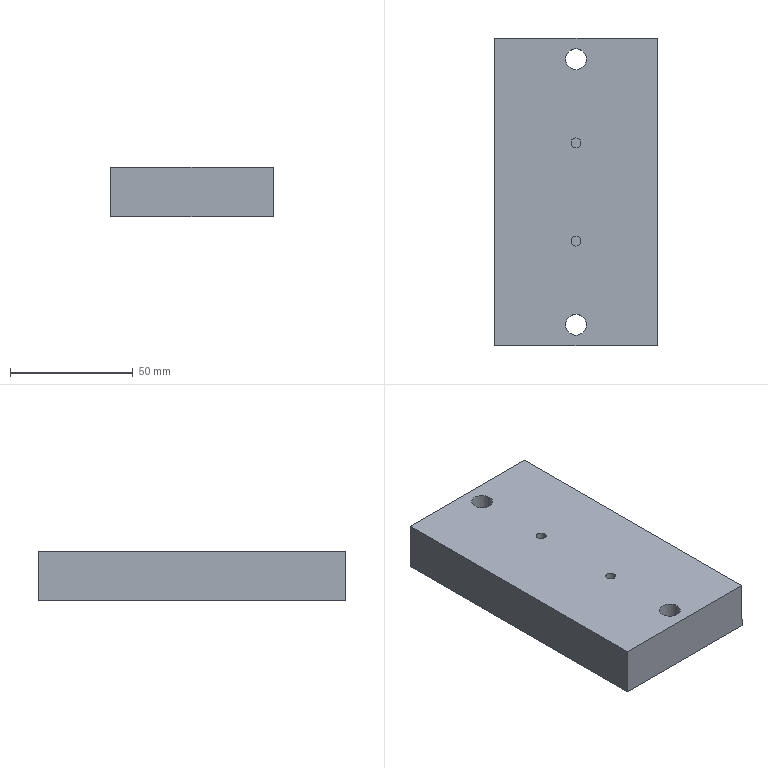NC program | NX | posted with a generic post | part box 65.936 x 125 x 20 mm
Lines 6200 to 6994 of 29196:
(PLANAR_MILL_2_COPY_COPY , TOOL : D10R0)
N12194 T10 M6
N12196 G54
N12198 G17 G0 G90 X-53.462 Y34.647 S4000 M3
N12200 G43 Z30. H10
N12202 G94 G1 Z-13.425 F5000.
N12204 G41 X-51. Y34.213 F1000. D10
N12206 X-45.
N12208 X45.
N12210 X51.
N12212 G40
N12214 X53.462 Y34.647
N12216 G0 Z5.
N12218 X-53.462
N12220 G1 Z-13.425 F5000.
N12222 G41 X-51. Y34.213 F1000.
N12224 X-45.
N12226 X45.
N12228 X51.
N12230 G40
N12232 X53.462 Y34.647
N12234 G0 Z5.
N12236 X-53.462
N12238 G1 Z-13.425 F5000.
N12240 G41 X-51. Y34.213 F1000.
N12242 X-45.
N12244 X45.
N12246 X51.
N12248 G40
N12250 X53.462 Y34.647
N12252 G0 Z30.
(FACE_MILLING_1 , TOOL : D10R0)
N12254 X51.7 Y-39.368
N12256 G1 Z-13.375 F5000.
N12258 X49.7 F1500.
N12260 X-49.7
N12262 Y-32.756
N12264 X49.7
N12266 Y-26.143
N12268 X-49.7
N12270 Y-19.531
N12272 X49.7
N12274 Y-12.918
N12276 X-49.7
N12278 X-51.7
N12280 G0 Z30.
N12282 X51.7 Y-39.386
N12284 G1 Z-13.425 F5000.
N12286 X49.7 F1500.
N12288 X-49.7
N12290 Y-32.792
N12292 X49.7
N12294 Y-26.198
N12296 X-49.7
N12298 Y-19.604
N12300 X49.7
N12302 Y-13.01
N12304 X-49.7
N12306 X-51.7
N12308 G0 Z30.
(FACE_MILLING_1_COPY_2 , TOOL : D10R0)
N12310 X51.7 Y-22.448
N12312 Z27.756
N12314 G1 Y-3.634 Z-11.253 F5000.
N12316 X49.7 F1500.
N12318 X-49.7
N12320 Y1.898 Z-8.585
N12322 X49.7
N12324 Y7.43 Z-5.917
N12326 X-49.7
N12328 Y12.961 Z-3.249
N12330 X49.7
N12332 Y18.493 Z-0.581
N12334 X-49.7
N12336 X-51.7
N12338 G0 Y-0.321 Z38.428
N12340 X51.7 Y-22.366 Z27.796
N12342 G1 Y-3.53 Z-11.258 F5000.
N12344 X49.7 F1500.
N12346 X-49.7
N12348 Y1.985 Z-8.598
N12350 X49.7
N12352 Y7.501 Z-5.938
N12354 X-49.7
N12356 Y13.016 Z-3.278
N12358 X49.7
N12360 Y18.531 Z-0.618
N12362 X-49.7
N12364 X-51.7
N12366 G0 Y-0.305 Z38.436
(PLANAR_MILL_2_COPY_COPY_1 , TOOL : D10R0)
N12368 X-25.525 Y55.553
N12370 Z7.259
N12372 G1 Y31.388 Z-9.661 F5000.
N12374 X-25.578 Y31.286 Z-9.527 F1500.
N12376 X-25.64 Y31.021 Z-9.178
N12378 Y30.82 Z-8.914
N12380 X-25.578 Y30.556 Z-8.566
N12382 X-25.447 Y30.3 Z-8.23
N12384 X-25.249 Y30.059 Z-7.916
N12386 X-24.991 Y29.84 Z-7.632
N12388 X-24.679 Y29.647 Z-7.386
N12390 X-24.32 Y29.485 Z-7.184
N12392 X-23.925 Y29.358 Z-7.032
N12394 X-23.503 Y29.268 Z-6.934
N12396 X-23.066 Y29.219 Z-6.893
N12398 X-22.734 Y29.208 Z-6.9
N12400 X-22.297 Y29.23 Z-6.961
N12402 X-21.875 Y29.291 Z-7.078
N12404 X-21.48 Y29.391 Z-7.25
N12406 X-21.121 Y29.525 Z-7.471
N12408 X-20.809 Y29.69 Z-7.737
N12410 X-20.551 Y29.882 Z-8.04
N12412 X-20.353 Y30.095 Z-8.374
N12414 X-20.222 Y30.323 Z-8.729
N12416 X-20.16 Y30.56 Z-9.097
N12418 Y30.739 Z-9.375
N12420 X-20.222 Y30.976 Z-9.743
N12422 X-20.353 Y31.204 Z-10.099
N12424 X-20.551 Y31.417 Z-10.432
N12426 X-20.809 Y31.609 Z-10.736
N12428 X-21.121 Y31.774 Z-11.001
N12430 X-21.48 Y31.908 Z-11.223
N12432 X-21.875 Y32.008 Z-11.394
N12434 X-22.297 Y32.069 Z-11.511
N12436 X-22.734 Y32.091 Z-11.572
N12438 X-23.066 Y32.08 Z-11.579
N12440 X-23.503 Y32.031 Z-11.538
N12442 X-23.925 Y31.942 Z-11.44
N12444 X-24.32 Y31.815 Z-11.288
N12446 X-24.679 Y31.653 Z-11.086
N12448 X-24.991 Y31.459 Z-10.84
N12450 X-25.249 Y31.24 Z-10.556
N12452 X-25.447 Y30.999 Z-10.242
N12454 X-25.578 Y30.743 Z-9.907
N12456 X-25.64 Y30.479 Z-9.558
N12458 Y30.278 Z-9.294
N12460 X-25.578 Y30.014 Z-8.945
N12462 X-25.447 Y29.758 Z-8.61
N12464 X-25.249 Y29.517 Z-8.296
N12466 X-24.991 Y29.298 Z-8.012
N12468 X-24.679 Y29.104 Z-7.766
N12470 X-24.32 Y28.942 Z-7.564
N12472 X-23.925 Y28.815 Z-7.412
N12474 X-23.503 Y28.726 Z-7.314
N12476 X-23.066 Y28.677 Z-7.273
N12478 X-22.734 Y28.666 Z-7.28
N12480 X-22.297 Y28.688 Z-7.341
N12482 X-21.875 Y28.749 Z-7.458
N12484 X-21.48 Y28.849 Z-7.629
N12486 X-21.121 Y28.983 Z-7.851
N12488 X-20.809 Y29.148 Z-8.116
N12490 X-20.551 Y29.34 Z-8.42
N12492 X-20.353 Y29.553 Z-8.753
N12494 X-20.222 Y29.781 Z-9.108
N12496 X-20.16 Y30.018 Z-9.476
N12498 Y30.197 Z-9.755
N12500 X-20.222 Y30.434 Z-10.123
N12502 X-20.353 Y30.662 Z-10.478
N12504 X-20.551 Y30.875 Z-10.812
N12506 X-20.809 Y31.067 Z-11.115
N12508 X-21.121 Y31.232 Z-11.381
N12510 X-21.48 Y31.366 Z-11.602
N12512 X-21.875 Y31.466 Z-11.774
N12514 X-22.297 Y31.527 Z-11.891
N12516 X-22.734 Y31.549 Z-11.952
N12518 X-23.066 Y31.538 Z-11.959
N12520 X-23.503 Y31.489 Z-11.918
N12522 X-23.925 Y31.399 Z-11.82
N12524 X-24.32 Y31.272 Z-11.668
N12526 X-24.679 Y31.11 Z-11.466
N12528 X-24.991 Y30.917 Z-11.22
N12530 X-25.249 Y30.698 Z-10.936
N12532 X-25.447 Y30.457 Z-10.622
N12534 X-25.578 Y30.201 Z-10.286
N12536 X-25.64 Y29.937 Z-9.938
N12538 Y29.736 Z-9.674
N12540 X-25.578 Y29.471 Z-9.325
N12542 X-25.447 Y29.215 Z-8.989
N12544 X-25.249 Y28.975 Z-8.675
N12546 X-24.991 Y28.755 Z-8.391
N12548 X-24.679 Y28.562 Z-8.145
N12550 X-24.32 Y28.4 Z-7.943
N12552 X-23.925 Y28.273 Z-7.791
N12554 X-23.503 Y28.184 Z-7.693
N12556 X-23.066 Y28.134 Z-7.652
N12558 X-22.734 Y28.124 Z-7.66
N12560 X-22.297 Y28.146 Z-7.72
N12562 X-21.875 Y28.207 Z-7.838
N12564 X-21.48 Y28.306 Z-8.009
N12566 X-21.121 Y28.441 Z-8.23
N12568 X-20.809 Y28.606 Z-8.496
N12570 X-20.551 Y28.798 Z-8.799
N12572 X-20.353 Y29.01 Z-9.133
N12574 X-20.222 Y29.238 Z-9.488
N12576 X-20.16 Y29.475 Z-9.856
N12578 Y29.655 Z-10.135
N12580 X-20.222 Y29.892 Z-10.503
N12582 X-20.353 Y30.12 Z-10.858
N12584 X-20.551 Y30.333 Z-11.192
N12586 X-20.809 Y30.525 Z-11.495
N12588 X-21.121 Y30.69 Z-11.761
N12590 X-21.48 Y30.824 Z-11.982
N12592 X-21.875 Y30.923 Z-12.153
N12594 X-22.297 Y30.985 Z-12.271
N12596 X-22.734 Y31.006 Z-12.331
N12598 X-23.066 Y30.996 Z-12.338
N12600 X-23.503 Y30.947 Z-12.297
N12602 X-23.925 Y30.857 Z-12.199
N12604 X-24.32 Y30.73 Z-12.047
N12606 X-24.679 Y30.568 Z-11.846
N12608 X-24.991 Y30.375 Z-11.6
N12610 X-25.249 Y30.156 Z-11.316
N12612 X-25.447 Y29.915 Z-11.002
N12614 X-25.578 Y29.659 Z-10.666
N12616 X-25.64 Y29.394 Z-10.317
N12618 Y29.194 Z-10.053
N12620 X-25.578 Y28.929 Z-9.705
N12622 X-25.447 Y28.673 Z-9.369
N12624 X-25.249 Y28.433 Z-9.055
N12626 X-24.991 Y28.213 Z-8.771
N12628 X-24.679 Y28.02 Z-8.525
N12630 X-24.32 Y27.858 Z-8.323
N12632 X-23.925 Y27.731 Z-8.171
N12634 X-23.503 Y27.642 Z-8.073
N12636 X-23.066 Y27.592 Z-8.032
N12638 X-22.734 Y27.582 Z-8.039
N12640 X-22.297 Y27.603 Z-8.1
N12642 X-21.875 Y27.665 Z-8.217
N12644 X-21.48 Y27.764 Z-8.389
N12646 X-21.121 Y27.898 Z-8.61
N12648 X-20.809 Y28.064 Z-8.876
N12650 X-20.551 Y28.255 Z-9.179
N12652 X-20.353 Y28.468 Z-9.512
N12654 X-20.222 Y28.696 Z-9.868
N12656 X-20.16 Y28.933 Z-10.236
N12658 Y29.113 Z-10.514
N12660 X-20.222 Y29.35 Z-10.882
N12662 X-20.353 Y29.578 Z-11.238
N12664 X-20.551 Y29.791 Z-11.571
N12666 X-20.809 Y29.982 Z-11.875
N12668 X-21.121 Y30.148 Z-12.14
N12670 X-21.48 Y30.282 Z-12.361
N12672 X-21.875 Y30.381 Z-12.533
N12674 X-22.297 Y30.443 Z-12.65
N12676 X-22.734 Y30.464 Z-12.711
N12678 X-23.066 Y30.454 Z-12.718
N12680 X-23.503 Y30.404 Z-12.677
N12682 X-23.925 Y30.315 Z-12.579
N12684 X-24.32 Y30.188 Z-12.427
N12686 X-24.679 Y30.026 Z-12.225
N12688 X-24.991 Y29.833 Z-11.979
N12690 X-25.249 Y29.613 Z-11.695
N12692 X-25.447 Y29.373 Z-11.381
N12694 X-25.578 Y29.117 Z-11.045
N12696 X-25.64 Y28.852 Z-10.697
N12698 Y28.652 Z-10.433
N12700 X-25.578 Y28.387 Z-10.084
N12702 X-25.447 Y28.131 Z-9.749
N12704 X-25.249 Y27.891 Z-9.435
N12706 X-24.991 Y27.671 Z-9.151
N12708 X-24.679 Y27.478 Z-8.904
N12710 X-24.32 Y27.316 Z-8.703
N12712 X-23.925 Y27.189 Z-8.551
N12714 X-23.503 Y27.1 Z-8.453
N12716 X-23.066 Y27.05 Z-8.412
N12718 X-22.734 Y27.04 Z-8.419
N12720 X-22.297 Y27.061 Z-8.48
N12722 X-21.875 Y27.123 Z-8.597
N12724 X-21.48 Y27.222 Z-8.768
N12726 X-21.121 Y27.356 Z-8.99
N12728 X-20.809 Y27.522 Z-9.255
N12730 X-20.551 Y27.713 Z-9.559
N12732 X-20.353 Y27.926 Z-9.892
N12734 X-20.222 Y28.154 Z-10.247
N12736 X-20.16 Y28.391 Z-10.615
N12738 Y28.571 Z-10.894
N12740 X-20.222 Y28.808 Z-11.262
N12742 X-20.353 Y29.036 Z-11.617
N12744 X-20.551 Y29.248 Z-11.951
N12746 X-20.809 Y29.44 Z-12.254
N12748 X-21.121 Y29.605 Z-12.52
N12750 X-21.48 Y29.74 Z-12.741
N12752 X-21.875 Y29.839 Z-12.912
N12754 X-22.297 Y29.9 Z-13.03
N12756 X-22.734 Y29.922 Z-13.09
N12758 X-23.066 Y29.912 Z-13.098
N12760 X-23.503 Y29.862 Z-13.057
N12762 X-23.925 Y29.773 Z-12.959
N12764 X-24.32 Y29.646 Z-12.807
N12766 X-24.679 Y29.484 Z-12.605
N12768 X-24.991 Y29.291 Z-12.359
N12770 X-25.249 Y29.071 Z-12.075
N12772 X-25.447 Y28.831 Z-11.761
N12774 X-25.578 Y28.575 Z-11.425
N12776 X-25.64 Y28.31 Z-11.077
N12778 Y28.11 Z-10.813
N12780 X-25.578 Y27.845 Z-10.464
N12782 X-25.447 Y27.589 Z-10.128
N12784 X-25.249 Y27.348 Z-9.814
N12786 X-24.991 Y27.129 Z-9.53
N12788 X-24.679 Y26.936 Z-9.284
N12790 X-24.32 Y26.774 Z-9.082
N12792 X-23.925 Y26.647 Z-8.93
N12794 X-23.503 Y26.557 Z-8.832
N12796 X-23.066 Y26.508 Z-8.791
N12798 X-22.734 Y26.497 Z-8.799
N12800 X-22.297 Y26.519 Z-8.859
N12802 X-21.875 Y26.581 Z-8.977
N12804 X-21.48 Y26.68 Z-9.148
N12806 X-21.121 Y26.814 Z-9.369
N12808 X-20.809 Y26.979 Z-9.635
N12810 X-20.551 Y27.171 Z-9.938
N12812 X-20.353 Y27.384 Z-10.272
N12814 X-20.222 Y27.612 Z-10.627
N12816 X-20.16 Y27.849 Z-10.995
N12818 Y28.028 Z-11.274
N12820 X-20.222 Y28.265 Z-11.642
N12822 X-20.353 Y28.493 Z-11.997
N12824 X-20.551 Y28.706 Z-12.33
N12826 X-20.809 Y28.898 Z-12.634
N12828 X-21.121 Y29.063 Z-12.899
N12830 X-21.48 Y29.197 Z-13.121
N12832 X-21.875 Y29.297 Z-13.292
N12834 X-22.297 Y29.358 Z-13.41
N12836 X-22.734 Y29.38 Z-13.47
N12838 X-23.066 Y29.37 Z-13.477
N12840 X-23.503 Y29.32 Z-13.436
N12842 X-23.925 Y29.231 Z-13.338
N12844 X-24.32 Y29.104 Z-13.186
N12846 X-24.679 Y28.942 Z-12.985
N12848 X-24.991 Y28.749 Z-12.738
N12850 X-25.249 Y28.529 Z-12.455
N12852 X-25.447 Y28.288 Z-12.141
N12854 X-25.578 Y28.033 Z-11.805
N12856 X-25.64 Y27.768 Z-11.456
N12858 Y27.567 Z-11.192
N12860 X-25.578 Y27.303 Z-10.844
N12862 X-25.447 Y27.047 Z-10.508
N12864 X-25.249 Y26.806 Z-10.194
N12866 X-24.991 Y26.587 Z-9.91
N12868 X-24.679 Y26.394 Z-9.664
N12870 X-24.32 Y26.232 Z-9.462
N12872 X-23.925 Y26.104 Z-9.31
N12874 X-23.503 Y26.015 Z-9.212
N12876 X-23.066 Y25.966 Z-9.171
N12878 X-22.734 Y25.955 Z-9.178
N12880 X-22.297 Y25.977 Z-9.239
N12882 X-21.875 Y26.038 Z-9.356
N12884 X-21.48 Y26.138 Z-9.528
N12886 X-21.121 Y26.272 Z-9.749
N12888 X-20.809 Y26.437 Z-10.015
N12890 X-20.551 Y26.629 Z-10.318
N12892 X-20.353 Y26.842 Z-10.651
N12894 X-20.222 Y27.07 Z-11.007
N12896 X-20.16 Y27.307 Z-11.375
N12898 Y27.486 Z-11.653
N12900 X-20.222 Y27.723 Z-12.021
N12902 X-20.353 Y27.951 Z-12.377
N12904 X-20.551 Y28.164 Z-12.71
N12906 X-20.809 Y28.356 Z-13.013
N12908 X-21.121 Y28.521 Z-13.279
N12910 X-21.48 Y28.655 Z-13.5
N12912 X-21.875 Y28.755 Z-13.672
N12914 X-22.297 Y28.816 Z-13.789
N12916 X-22.734 Y28.838 Z-13.85
N12918 X-23.066 Y28.827 Z-13.857
N12920 X-23.503 Y28.778 Z-13.816
N12922 X-23.925 Y28.689 Z-13.718
N12924 X-24.32 Y28.561 Z-13.566
N12926 X-24.679 Y28.399 Z-13.364
N12928 X-24.991 Y28.206 Z-13.118
N12930 X-25.249 Y27.987 Z-12.834
N12932 X-25.447 Y27.746 Z-12.52
N12934 X-25.578 Y27.49 Z-12.184
N12936 X-25.64 Y27.226 Z-11.836
N12938 Y27.025 Z-11.572
N12940 X-25.578 Y26.76 Z-11.223
N12942 X-25.447 Y26.505 Z-10.887
N12944 X-25.249 Y26.264 Z-10.573
N12946 X-24.991 Y26.044 Z-10.29
N12948 X-24.679 Y25.851 Z-10.043
N12950 X-24.32 Y25.689 Z-9.842
N12952 X-23.925 Y25.562 Z-9.69
N12954 X-23.503 Y25.473 Z-9.592
N12956 X-23.066 Y25.423 Z-9.551
N12958 X-22.734 Y25.413 Z-9.558
N12960 X-22.297 Y25.435 Z-9.618
N12962 X-21.875 Y25.496 Z-9.736
N12964 X-21.48 Y25.596 Z-9.907
N12966 X-21.121 Y25.73 Z-10.129
N12968 X-20.809 Y25.895 Z-10.394
N12970 X-20.551 Y26.087 Z-10.698
N12972 X-20.353 Y26.3 Z-11.031
N12974 X-20.222 Y26.528 Z-11.386
N12976 X-20.16 Y26.765 Z-11.754
N12978 Y26.944 Z-12.033
N12980 X-20.222 Y27.181 Z-12.401
N12982 X-20.353 Y27.409 Z-12.756
N12984 X-20.551 Y27.622 Z-13.09
N12986 X-20.809 Y27.814 Z-13.393
N12988 X-21.121 Y27.979 Z-13.659
N12990 X-21.48 Y28.113 Z-13.88
N12992 X-21.875 Y28.212 Z-14.051
N12994 X-22.297 Y28.274 Z-14.169
N12996 X-22.734 Y28.296 Z-14.229
N12998 X-23.066 Y28.285 Z-14.237
N13000 X-23.503 Y28.236 Z-14.196
N13002 X-23.925 Y28.146 Z-14.098
N13004 X-24.32 Y28.019 Z-13.946
N13006 X-24.679 Y27.857 Z-13.744
N13008 X-24.991 Y27.664 Z-13.498
N13010 X-25.249 Y27.445 Z-13.214
N13012 X-25.447 Y27.204 Z-12.9
N13014 X-25.578 Y26.948 Z-12.564
N13016 X-25.64 Y26.683 Z-12.215
N13018 Y26.483 Z-11.951
N13020 X-25.578 Y26.218 Z-11.603
N13022 X-25.447 Y25.962 Z-11.267
N13024 X-25.249 Y25.722 Z-10.953
N13026 X-24.991 Y25.502 Z-10.669
N13028 X-24.679 Y25.309 Z-10.423
N13030 X-24.32 Y25.147 Z-10.221
N13032 X-23.925 Y25.02 Z-10.069
N13034 X-23.503 Y24.931 Z-9.971
N13036 X-23.066 Y24.881 Z-9.93
N13038 X-22.734 Y24.871 Z-9.938
N13040 X-22.297 Y24.893 Z-9.998
N13042 X-21.875 Y24.954 Z-10.115
N13044 X-21.48 Y25.053 Z-10.287
N13046 X-21.121 Y25.188 Z-10.508
N13048 X-20.809 Y25.353 Z-10.774
N13050 X-20.551 Y25.545 Z-11.077
N13052 X-20.353 Y25.757 Z-11.411
N13054 X-20.222 Y25.985 Z-11.766
N13056 X-20.16 Y26.222 Z-12.134
N13058 Y26.402 Z-12.413
N13060 X-20.222 Y26.639 Z-12.781
N13062 X-20.353 Y26.867 Z-13.136
N13064 X-20.551 Y27.08 Z-13.469
N13066 X-20.809 Y27.271 Z-13.773
N13068 X-21.121 Y27.437 Z-14.038
N13070 X-21.48 Y27.571 Z-14.26
N13072 X-21.875 Y27.67 Z-14.431
N13074 X-22.297 Y27.732 Z-14.548
N13076 X-22.734 Y27.753 Z-14.609
N13078 X-23.066 Y27.743 Z-14.616
N13080 X-23.503 Y27.693 Z-14.575
N13082 X-23.925 Y27.604 Z-14.477
N13084 X-24.32 Y27.477 Z-14.325
N13086 X-24.679 Y27.315 Z-14.124
N13088 X-24.991 Y27.122 Z-13.877
N13090 X-25.249 Y26.902 Z-13.593
N13092 X-25.447 Y26.662 Z-13.279
N13094 X-25.578 Y26.406 Z-12.944
N13096 X-25.64 Y26.141 Z-12.595
N13098 Y25.941 Z-12.331
N13100 X-25.578 Y25.676 Z-11.983
N13102 X-25.447 Y25.42 Z-11.647
N13104 X-25.249 Y25.18 Z-11.333
N13106 X-24.991 Y24.96 Z-11.049
N13108 X-24.679 Y24.767 Z-10.803
N13110 X-24.32 Y24.605 Z-10.601
N13112 X-23.925 Y24.478 Z-10.449
N13114 X-23.503 Y24.389 Z-10.351
N13116 X-23.066 Y24.339 Z-10.31
N13118 X-22.734 Y24.329 Z-10.317
N13120 X-22.297 Y24.35 Z-10.378
N13122 X-21.875 Y24.412 Z-10.495
N13124 X-21.48 Y24.511 Z-10.667
N13126 X-21.121 Y24.645 Z-10.888
N13128 X-20.809 Y24.811 Z-11.153
N13130 X-20.551 Y25.002 Z-11.457
N13132 X-20.353 Y25.215 Z-11.79
N13134 X-20.222 Y25.443 Z-12.146
N13136 X-20.16 Y25.68 Z-12.514
N13138 Y25.86 Z-12.792
N13140 X-20.222 Y26.097 Z-13.16
N13142 X-20.353 Y26.325 Z-13.516
N13144 X-20.551 Y26.538 Z-13.849
N13146 X-20.809 Y26.729 Z-14.152
N13148 X-21.121 Y26.895 Z-14.418
N13150 X-21.48 Y27.029 Z-14.639
N13152 X-21.875 Y27.128 Z-14.811
N13154 X-22.297 Y27.19 Z-14.928
N13156 X-22.734 Y27.211 Z-14.989
N13158 X-23.066 Y27.201 Z-14.996
N13160 X-23.503 Y27.151 Z-14.955
N13162 X-23.925 Y27.062 Z-14.857
N13164 X-24.32 Y26.935 Z-14.705
N13166 X-24.679 Y26.773 Z-14.503
N13168 X-24.991 Y26.58 Z-14.257
N13170 X-25.249 Y26.36 Z-13.973
N13172 X-25.447 Y26.12 Z-13.659
N13174 X-25.578 Y25.864 Z-13.323
N13176 X-25.64 Y25.599 Z-12.975
N13178 Y25.399 Z-12.711
N13180 X-25.578 Y25.134 Z-12.362
N13182 X-25.447 Y24.878 Z-12.026
N13184 X-25.249 Y24.637 Z-11.712
N13186 X-24.991 Y24.418 Z-11.428
N13188 X-24.679 Y24.225 Z-11.182
N13190 X-24.32 Y24.063 Z-10.98
N13192 X-23.925 Y23.936 Z-10.829
N13194 X-23.503 Y23.846 Z-10.731
N13196 X-23.066 Y23.797 Z-10.69
N13198 X-22.734 Y23.786 Z-10.697
N13200 X-22.297 Y23.808 Z-10.757
N13202 X-21.875 Y23.87 Z-10.875
N13204 X-21.48 Y23.969 Z-11.046
N13206 X-21.121 Y24.103 Z-11.267
N13208 X-20.809 Y24.268 Z-11.533
N13210 X-20.551 Y24.46 Z-11.836
N13212 X-20.353 Y24.673 Z-12.17
N13214 X-20.222 Y24.901 Z-12.525
N13216 X-20.16 Y25.138 Z-12.893
N13218 Y25.318 Z-13.172
N13220 X-20.222 Y25.555 Z-13.54
N13222 X-20.353 Y25.783 Z-13.895
N13224 X-20.551 Y25.995 Z-14.229
N13226 X-20.809 Y26.187 Z-14.532
N13228 X-21.121 Y26.352 Z-14.798
N13230 X-21.48 Y26.487 Z-15.019
N13232 X-21.875 Y26.586 Z-15.19
N13234 X-22.297 Y26.647 Z-15.308
N13236 X-22.734 Y26.669 Z-15.368
N13238 X-23.066 Y26.659 Z-15.376
N13240 X-23.503 Y26.609 Z-15.334
N13242 X-23.925 Y26.52 Z-15.237
N13244 X-24.32 Y26.393 Z-15.085
N13246 X-24.679 Y26.231 Z-14.883
N13248 X-24.991 Y26.038 Z-14.637
N13250 X-25.249 Y25.818 Z-14.353
N13252 X-25.447 Y25.577 Z-14.039
N13254 X-25.578 Y25.322 Z-13.703
N13256 X-25.64 Y25.057 Z-13.354
N13258 Y24.856 Z-13.09
N13260 X-25.578 Y24.592 Z-12.742
N13262 X-25.447 Y24.336 Z-12.406
N13264 X-25.249 Y24.095 Z-12.092
N13266 X-24.991 Y23.876 Z-11.808
N13268 X-24.679 Y23.683 Z-11.562
N13270 X-24.32 Y23.521 Z-11.36
N13272 X-23.925 Y23.394 Z-11.208
N13274 X-23.503 Y23.304 Z-11.11
N13276 X-23.066 Y23.255 Z-11.069
N13278 X-22.734 Y23.244 Z-11.076
N13280 X-22.297 Y23.266 Z-11.137
N13282 X-21.875 Y23.327 Z-11.254
N13284 X-21.48 Y23.427 Z-11.426
N13286 X-21.121 Y23.561 Z-11.647
N13288 X-20.809 Y23.726 Z-11.913
N13290 X-20.551 Y23.918 Z-12.216
N13292 X-20.353 Y24.131 Z-12.55
N13294 X-20.222 Y24.359 Z-12.905
N13296 X-20.16 Y24.596 Z-13.273
N13298 Y24.775 Z-13.551
N13300 X-20.222 Y25.012 Z-13.92
N13302 X-20.353 Y25.24 Z-14.275
N13304 X-20.551 Y25.453 Z-14.608
N13306 X-20.809 Y25.645 Z-14.912
N13308 X-21.121 Y25.81 Z-15.177
N13310 X-21.48 Y25.944 Z-15.399
N13312 X-21.875 Y26.044 Z-15.57
N13314 X-22.297 Y26.105 Z-15.687
N13316 X-22.734 Y26.127 Z-15.748
N13318 X-23.066 Y26.116 Z-15.755
N13320 X-23.503 Y26.067 Z-15.714
N13322 X-23.925 Y25.978 Z-15.616
N13324 X-24.32 Y25.851 Z-15.464
N13326 X-24.679 Y25.689 Z-15.262
N13328 X-24.991 Y25.495 Z-15.016
N13330 X-25.249 Y25.276 Z-14.732
N13332 X-25.447 Y25.035 Z-14.418
N13334 X-25.578 Y24.779 Z-14.083
N13336 X-25.64 Y24.515 Z-13.734
N13338 Y24.314 Z-13.47
N13340 X-25.578 Y24.049 Z-13.121
N13342 X-25.447 Y23.794 Z-12.786
N13344 X-25.249 Y23.553 Z-12.472
N13346 X-24.991 Y23.334 Z-12.188
N13348 X-24.679 Y23.14 Z-11.942
N13350 X-24.32 Y22.978 Z-11.74
N13352 X-23.925 Y22.851 Z-11.588
N13354 X-23.503 Y22.762 Z-11.49
N13356 X-23.066 Y22.713 Z-11.449
N13358 X-22.734 Y22.702 Z-11.456
N13360 X-22.297 Y22.724 Z-11.517
N13362 X-21.875 Y22.785 Z-11.634
N13364 X-21.48 Y22.885 Z-11.805
N13366 X-21.121 Y23.019 Z-12.027
N13368 X-20.809 Y23.184 Z-12.292
N13370 X-20.551 Y23.376 Z-12.596
N13372 X-20.353 Y23.589 Z-12.929
N13374 X-20.222 Y23.817 Z-13.284
N13376 X-20.16 Y24.054 Z-13.653
N13378 Y24.233 Z-13.931
N13380 X-20.222 Y24.47 Z-14.299
N13382 X-20.353 Y24.698 Z-14.654
N13384 X-20.551 Y24.911 Z-14.988
N13386 X-20.809 Y25.103 Z-15.291
N13388 X-21.121 Y25.268 Z-15.557
N13390 X-21.48 Y25.402 Z-15.778
N13392 X-21.875 Y25.501 Z-15.95
N13394 X-22.297 Y25.563 Z-16.067
N13396 X-22.734 Y25.585 Z-16.128
N13398 X-23.066 Y25.574 Z-16.135
N13400 X-23.503 Y25.525 Z-16.094
N13402 X-23.925 Y25.435 Z-15.996
N13404 X-24.32 Y25.308 Z-15.844
N13406 X-24.679 Y25.146 Z-15.642
N13408 X-24.991 Y24.953 Z-15.396
N13410 X-25.249 Y24.734 Z-15.112
N13412 X-25.447 Y24.493 Z-14.798
N13414 X-25.578 Y24.237 Z-14.462
N13416 X-25.64 Y23.972 Z-14.114
N13418 Y23.772 Z-13.85
N13420 X-25.578 Y23.507 Z-13.501
N13422 X-25.447 Y23.251 Z-13.165
N13424 X-25.249 Y23.011 Z-12.851
N13426 X-24.991 Y22.791 Z-12.567
N13428 X-24.679 Y22.598 Z-12.321
N13430 X-24.32 Y22.436 Z-12.119
N13432 X-23.925 Y22.309 Z-11.967
N13434 X-23.503 Y22.22 Z-11.87
N13436 X-23.066 Y22.17 Z-11.828
N13438 X-22.734 Y22.16 Z-11.836
N13440 X-22.297 Y22.182 Z-11.896
N13442 X-21.875 Y22.243 Z-12.014
N13444 X-21.48 Y22.342 Z-12.185
N13446 X-21.121 Y22.477 Z-12.406
N13448 X-20.809 Y22.642 Z-12.672
N13450 X-20.551 Y22.834 Z-12.975
N13452 X-20.353 Y23.046 Z-13.309
N13454 X-20.222 Y23.274 Z-13.664
N13456 X-20.16 Y23.511 Z-14.032
N13458 Y23.691 Z-14.311
N13460 X-20.222 Y23.928 Z-14.679
N13462 X-20.353 Y24.156 Z-15.034
N13464 X-20.551 Y24.369 Z-15.368
N13466 X-20.809 Y24.561 Z-15.671
N13468 X-21.121 Y24.726 Z-15.937
N13470 X-21.48 Y24.86 Z-16.158
N13472 X-21.875 Y24.959 Z-16.329
N13474 X-22.297 Y25.021 Z-16.447
N13476 X-22.734 Y25.042 Z-16.507
N13478 X-23.066 Y25.032 Z-16.515
N13480 X-23.503 Y24.983 Z-16.473
N13482 X-23.925 Y24.893 Z-16.375
N13484 X-24.32 Y24.766 Z-16.224
N13486 X-24.679 Y24.604 Z-16.022
N13488 X-24.991 Y24.411 Z-15.776
N13490 X-25.249 Y24.192 Z-15.492
N13492 X-25.447 Y23.951 Z-15.178
N13494 X-25.578 Y23.695 Z-14.842
N13496 X-25.64 Y23.43 Z-14.493
N13498 Y23.23 Z-14.229
N13500 X-25.578 Y22.965 Z-13.881
N13502 X-25.447 Y22.709 Z-13.545
N13504 X-25.249 Y22.469 Z-13.231
N13506 X-24.991 Y22.249 Z-12.947
N13508 X-24.679 Y22.056 Z-12.701
N13510 X-24.32 Y21.894 Z-12.499
N13512 X-23.925 Y21.767 Z-12.347
N13514 X-23.503 Y21.678 Z-12.249
N13516 X-23.066 Y21.628 Z-12.208
N13518 X-22.734 Y21.618 Z-12.215
N13520 X-22.297 Y21.639 Z-12.276
N13522 X-21.875 Y21.701 Z-12.393
N13524 X-21.48 Y21.8 Z-12.565
N13526 X-21.121 Y21.934 Z-12.786
N13528 X-20.809 Y22.1 Z-13.052
N13530 X-20.551 Y22.291 Z-13.355
N13532 X-20.353 Y22.504 Z-13.689
N13534 X-20.222 Y22.732 Z-14.044
N13536 X-20.16 Y22.969 Z-14.412
N13538 Y23.149 Z-14.69
N13540 X-20.222 Y23.386 Z-15.058
N13542 X-20.353 Y23.614 Z-15.414
N13544 X-20.551 Y23.827 Z-15.747
N13546 X-20.809 Y24.018 Z-16.051
N13548 X-21.121 Y24.184 Z-16.316
N13550 X-21.48 Y24.318 Z-16.537
N13552 X-21.875 Y24.417 Z-16.709
N13554 X-22.297 Y24.479 Z-16.826
N13556 X-22.734 Y24.5 Z-16.887
N13558 X-23.066 Y24.49 Z-16.894
N13560 X-23.503 Y24.44 Z-16.853
N13562 X-23.925 Y24.351 Z-16.755
N13564 X-24.32 Y24.224 Z-16.603
N13566 X-24.679 Y24.062 Z-16.401
N13568 X-24.991 Y23.869 Z-16.155
N13570 X-25.249 Y23.649 Z-15.871
N13572 X-25.447 Y23.409 Z-15.557
N13574 X-25.578 Y23.153 Z-15.222
N13576 X-25.64 Y22.888 Z-14.873
N13578 Y22.688 Z-14.609
N13580 X-25.578 Y22.423 Z-14.26
N13582 X-25.447 Y22.167 Z-13.925
N13584 X-25.249 Y21.927 Z-13.611
N13586 X-24.991 Y21.707 Z-13.327
N13588 X-24.679 Y21.514 Z-13.08
N13590 X-24.32 Y21.352 Z-12.879
N13592 X-23.925 Y21.225 Z-12.727
N13594 X-23.503 Y21.135 Z-12.629
N13596 X-23.066 Y21.086 Z-12.588
N13598 X-22.734 Y21.076 Z-12.595
N13600 X-22.297 Y21.097 Z-12.656
N13602 X-21.875 Y21.159 Z-12.773
N13604 X-21.48 Y21.258 Z-12.944
N13606 X-21.121 Y21.392 Z-13.166
N13608 X-20.809 Y21.558 Z-13.431
N13610 X-20.551 Y21.749 Z-13.735
N13612 X-20.353 Y21.962 Z-14.068
N13614 X-20.222 Y22.19 Z-14.423
N13616 X-20.16 Y22.427 Z-14.791
N13618 Y22.607 Z-15.07
N13620 X-20.222 Y22.844 Z-15.438
N13622 X-20.353 Y23.072 Z-15.793
N13624 X-20.551 Y23.284 Z-16.127
N13626 X-20.809 Y23.476 Z-16.43
N13628 X-21.121 Y23.641 Z-16.696
N13630 X-21.48 Y23.776 Z-16.917
N13632 X-21.875 Y23.875 Z-17.089
N13634 X-22.297 Y23.936 Z-17.206
N13636 X-22.734 Y23.958 Z-17.266
N13638 X-23.066 Y23.948 Z-17.274
N13640 X-23.503 Y23.898 Z-17.233
N13642 X-23.925 Y23.809 Z-17.135
N13644 X-24.32 Y23.682 Z-16.983
N13646 X-24.679 Y23.52 Z-16.781
N13648 X-24.991 Y23.327 Z-16.535
N13650 X-25.249 Y23.107 Z-16.251
N13652 X-25.447 Y22.867 Z-15.937
N13654 X-25.578 Y22.611 Z-15.601
N13656 X-25.64 Y22.346 Z-15.253
N13658 Y22.146 Z-14.989
N13660 X-25.578 Y21.881 Z-14.64
N13662 X-25.447 Y21.625 Z-14.304
N13664 X-25.249 Y21.384 Z-13.99
N13666 X-24.991 Y21.165 Z-13.706
N13668 X-24.679 Y20.972 Z-13.46
N13670 X-24.32 Y20.81 Z-13.258
N13672 X-23.925 Y20.683 Z-13.106
N13674 X-23.503 Y20.593 Z-13.008
N13676 X-23.066 Y20.544 Z-12.967
N13678 X-22.734 Y20.533 Z-12.975
N13680 X-22.297 Y20.555 Z-13.035
N13682 X-21.875 Y20.617 Z-13.153
N13684 X-21.48 Y20.716 Z-13.324
N13686 X-21.121 Y20.85 Z-13.545
N13688 X-20.809 Y21.015 Z-13.811
N13690 X-20.551 Y21.207 Z-14.114
N13692 X-20.353 Y21.42 Z-14.448
N13694 X-20.222 Y21.648 Z-14.803
N13696 X-20.16 Y21.885 Z-15.171
N13698 Y22.064 Z-15.45
N13700 X-20.222 Y22.301 Z-15.818
N13702 X-20.353 Y22.529 Z-16.173
N13704 X-20.551 Y22.742 Z-16.506
N13706 X-20.809 Y22.934 Z-16.81
N13708 X-21.121 Y23.099 Z-17.075
N13710 X-21.48 Y23.233 Z-17.297
N13712 X-21.875 Y23.333 Z-17.468
N13714 X-22.297 Y23.394 Z-17.586
N13716 X-22.734 Y23.416 Z-17.646
N13718 X-23.066 Y23.405 Z-17.653
N13720 X-23.503 Y23.356 Z-17.612
N13722 X-23.925 Y23.267 Z-17.514
N13724 X-24.32 Y23.14 Z-17.362
N13726 X-24.679 Y22.978 Z-17.161
N13728 X-24.991 Y22.785 Z-16.915
N13730 X-25.249 Y22.565 Z-16.631
N13732 X-25.447 Y22.324 Z-16.317
N13734 X-25.578 Y22.069 Z-15.981
N13736 X-25.64 Y21.804 Z-15.632
N13738 Y21.603 Z-15.368
N13740 X-25.578 Y21.339 Z-15.02
N13742 X-25.447 Y21.083 Z-14.684
N13744 X-25.249 Y20.842 Z-14.37
N13746 X-24.991 Y20.623 Z-14.086
N13748 X-24.679 Y20.43 Z-13.84
N13750 X-24.32 Y20.268 Z-13.638
N13752 X-23.925 Y20.14 Z-13.486
N13754 X-23.503 Y20.051 Z-13.388
N13756 X-23.066 Y20.002 Z-13.347
N13758 X-22.734 Y19.991 Z-13.354